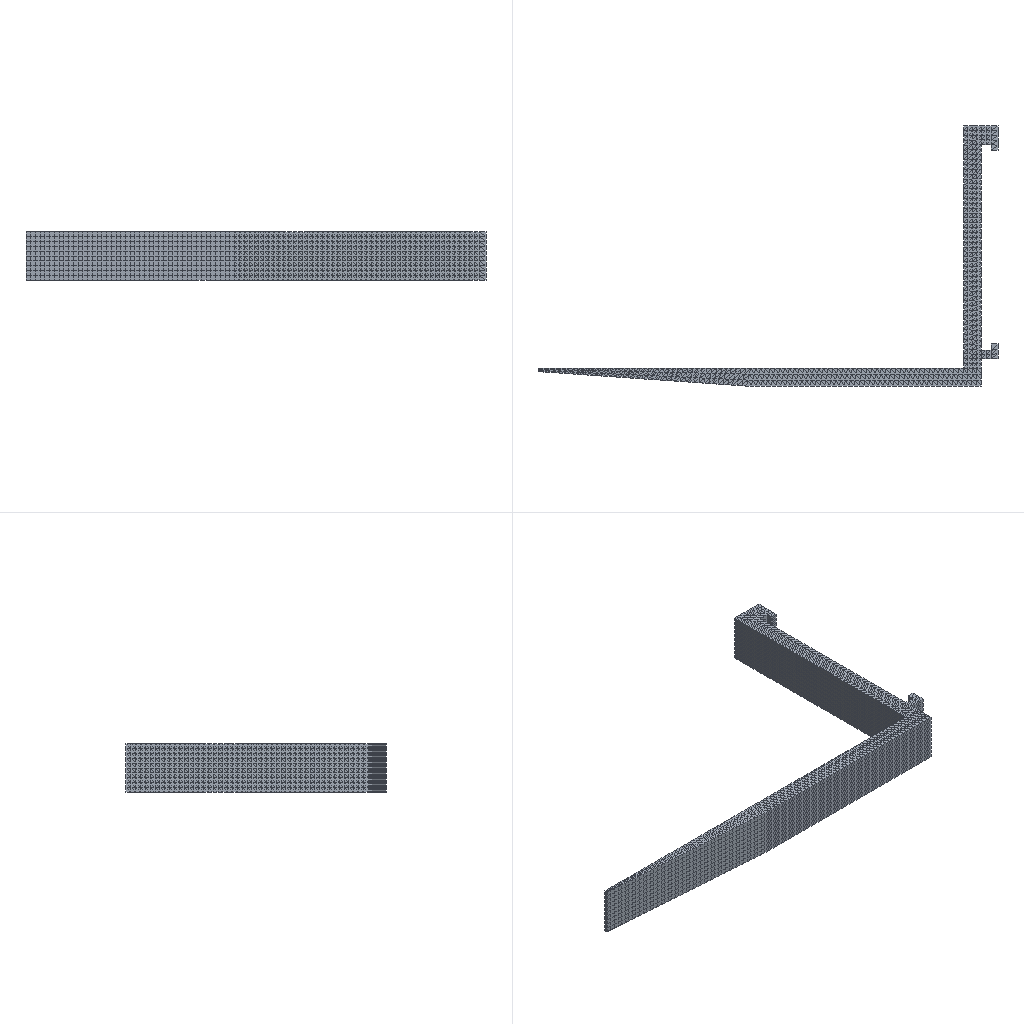Simulation study | abaqus
Set-up summary:
category,name,step,type,value,unit,region
solver,abaqus,,Abaqus/CAE 2024
units,mm-N-s-tonne (MPa),,inferred,E=240000 density=1.8e-09
analysis,Step-1,,dynamic explicit,nlgeom=True; time_period=1
mesh,nodes,,,7150
mesh,elements,,,8982
element_type,C3D8R,,,4960
element_type,S4R,,,4022
material,Material-CFRP,,E,240000
material,Material-CFRP,,nu,0.25
material,Material-CFRP,,density,1.8e-09
material,Material-CFRP,,behaviors,damage initiation; damage evolution; elastic lamina
material,Material-foam,,density,5.1e-11
section,Material-foam,,solid section,,,Set-31
section,,,shell section,0.2,,CompositeLayup-1-1
section,,,shell section,0.2,,CompositeLayup-2-1
load,Load-1,Step-1,pressure,0.1,,Surf-2
bc,BC-1,initial,encastre,[dofs=ENCASTRE],,Set-2
contact,Int-1,initial,general contact,interaction=IntProp-1; friction=0.15; behavior=hard
Abaqus input file, long lists of numbers shortened:
*Heading
** Job name: deck Model name: 0413
** Generated by: Abaqus/CAE 2024
*Preprint, echo=NO, model=NO, history=NO, contact=NO
**
** PARTS
**
*Part, name=huocha
*End Part
**
**
** ASSEMBLY
**
*Assembly, name=Assembly
**
*Instance, name=huocha-1, part=huocha
*Node
      1,        1118.,         598.,         120.
      2,        1118.,         598.,           0.
** (7148 more lines like these left out)
*Element, type=C3D8R
 1,   90,  861, 4172,  855,    1,   45,  837,   64
 2,  861,  862, 4173, 4172,   45,   46,  838,  837
** (4958 more lines like these left out)
*Element, type=S4R
4961,   5, 172,  18,  17
4962,  96, 173, 172,   5
** (4020 more lines like these left out)
*Nset, nset=_PickedSet5, internal
    1,    2,    3,    4,    5,    6,    7,    8,    9,   10,   11,   12,   13,   14,   15,   16
   17,   18,   19,   20,   21,   22,   23,   26,   27,   28,   29,   30,   31,   32,   33,   34
** (139 more lines like these left out)
*Elset, elset=_PickedSet5, internal
 4974, 4975, 4976, 4977, 4978, 4979, 4980, 4981, 4982, 4983, 4984, 4985, 4986, 4987, 4988, 4989
 4990, 4991, 4992, 4993, 4994, 4995, 4996, 4997, 4998, 4999, 5000, 5001, 5002, 5003, 5011, 5012
** (121 more lines like these left out)
*Nset, nset=_PickedSet6, internal
    1,    2,    3,    4,    5,    6,    7,    8,    9,   10,   11,   12,   13,   14,   15,   16
   17,   18,   19,   20,   21,   22,   23,   26,   27,   28,   29,   30,   31,   32,   33,   34
** (139 more lines like these left out)
*Elset, elset=_PickedSet6, internal
 4974, 4975, 4976, 4977, 4978, 4979, 4980, 4981, 4982, 4983, 4984, 4985, 4986, 4987, 4988, 4989
 4990, 4991, 4992, 4993, 4994, 4995, 4996, 4997, 4998, 4999, 5000, 5001, 5002, 5003, 5011, 5012
** (121 more lines like these left out)
*Nset, nset=_PickedSet7, internal
    1,    2,    3,    4,    5,    6,    7,    8,    9,   10,   11,   12,   13,   14,   15,   16
   17,   18,   19,   20,   21,   22,   23,   26,   27,   28,   29,   30,   31,   32,   33,   34
** (139 more lines like these left out)
*Elset, elset=_PickedSet7, internal
 4974, 4975, 4976, 4977, 4978, 4979, 4980, 4981, 4982, 4983, 4984, 4985, 4986, 4987, 4988, 4989
 4990, 4991, 4992, 4993, 4994, 4995, 4996, 4997, 4998, 4999, 5000, 5001, 5002, 5003, 5011, 5012
** (121 more lines like these left out)
*Nset, nset=_PickedSet8, internal
    1,    2,    3,    4,    5,    6,    7,    8,    9,   10,   11,   12,   13,   14,   15,   16
   17,   18,   19,   20,   21,   22,   23,   26,   27,   28,   29,   30,   31,   32,   33,   34
** (139 more lines like these left out)
*Elset, elset=_PickedSet8, internal
 4974, 4975, 4976, 4977, 4978, 4979, 4980, 4981, 4982, 4983, 4984, 4985, 4986, 4987, 4988, 4989
 4990, 4991, 4992, 4993, 4994, 4995, 4996, 4997, 4998, 4999, 5000, 5001, 5002, 5003, 5011, 5012
** (121 more lines like these left out)
*Nset, nset=_PickedSet9, internal
    1,    2,    3,    4,    5,    6,    7,    8,    9,   10,   11,   12,   13,   14,   15,   16
   17,   18,   19,   20,   21,   22,   23,   26,   27,   28,   29,   30,   31,   32,   33,   34
** (139 more lines like these left out)
*Elset, elset=_PickedSet9, internal
 4974, 4975, 4976, 4977, 4978, 4979, 4980, 4981, 4982, 4983, 4984, 4985, 4986, 4987, 4988, 4989
 4990, 4991, 4992, 4993, 4994, 4995, 4996, 4997, 4998, 4999, 5000, 5001, 5002, 5003, 5011, 5012
** (121 more lines like these left out)
*Nset, nset=_PickedSet10, internal
    1,    2,    3,    4,    5,    6,    7,    8,    9,   10,   11,   12,   13,   14,   15,   16
   17,   18,   19,   20,   21,   22,   23,   26,   27,   28,   29,   30,   31,   32,   33,   34
** (139 more lines like these left out)
*Elset, elset=_PickedSet10, internal
 4974, 4975, 4976, 4977, 4978, 4979, 4980, 4981, 4982, 4983, 4984, 4985, 4986, 4987, 4988, 4989
 4990, 4991, 4992, 4993, 4994, 4995, 4996, 4997, 4998, 4999, 5000, 5001, 5002, 5003, 5011, 5012
** (121 more lines like these left out)
*Nset, nset=_PickedSet11, internal
    1,    2,    3,    4,    5,    6,    7,    8,    9,   10,   11,   12,   13,   14,   15,   16
   17,   18,   19,   20,   21,   22,   23,   26,   27,   28,   29,   30,   31,   32,   33,   34
** (139 more lines like these left out)
*Elset, elset=_PickedSet11, internal
 4974, 4975, 4976, 4977, 4978, 4979, 4980, 4981, 4982, 4983, 4984, 4985, 4986, 4987, 4988, 4989
 4990, 4991, 4992, 4993, 4994, 4995, 4996, 4997, 4998, 4999, 5000, 5001, 5002, 5003, 5011, 5012
** (121 more lines like these left out)
*Nset, nset=_PickedSet12, internal
    1,    2,    3,    4,    5,    6,    7,    8,    9,   10,   11,   12,   13,   14,   15,   16
   17,   18,   19,   20,   21,   22,   23,   26,   27,   28,   29,   30,   31,   32,   33,   34
** (139 more lines like these left out)
*Elset, elset=_PickedSet12, internal
 4974, 4975, 4976, 4977, 4978, 4979, 4980, 4981, 4982, 4983, 4984, 4985, 4986, 4987, 4988, 4989
 4990, 4991, 4992, 4993, 4994, 4995, 4996, 4997, 4998, 4999, 5000, 5001, 5002, 5003, 5011, 5012
** (121 more lines like these left out)
*Nset, nset=_PickedSet13, internal
    1,    2,    3,    4,    5,    6,    7,    8,    9,   10,   11,   12,   13,   14,   15,   16
   17,   18,   19,   20,   21,   22,   23,   26,   27,   28,   29,   30,   31,   32,   33,   34
** (139 more lines like these left out)
*Elset, elset=_PickedSet13, internal
 4974, 4975, 4976, 4977, 4978, 4979, 4980, 4981, 4982, 4983, 4984, 4985, 4986, 4987, 4988, 4989
 4990, 4991, 4992, 4993, 4994, 4995, 4996, 4997, 4998, 4999, 5000, 5001, 5002, 5003, 5011, 5012
** (121 more lines like these left out)
*Nset, nset=_PickedSet14, internal
    1,    2,    3,    4,    5,    6,    7,    8,    9,   10,   11,   12,   13,   14,   15,   16
   17,   18,   19,   20,   21,   22,   23,   26,   27,   28,   29,   30,   31,   32,   33,   34
** (139 more lines like these left out)
*Elset, elset=_PickedSet14, internal
 4974, 4975, 4976, 4977, 4978, 4979, 4980, 4981, 4982, 4983, 4984, 4985, 4986, 4987, 4988, 4989
 4990, 4991, 4992, 4993, 4994, 4995, 4996, 4997, 4998, 4999, 5000, 5001, 5002, 5003, 5011, 5012
** (121 more lines like these left out)
*Nset, nset=_PickedSet15, internal
    1,    2,    3,    4,    5,    6,    7,    8,    9,   10,   11,   12,   13,   14,   15,   16
   17,   18,   19,   20,   21,   22,   23,   24,   25,   26,   27,   28,   29,   30,   31,   32
** (194 more lines like these left out)
*Elset, elset=_PickedSet15, internal, generate
 4961,  7912,     1
*Nset, nset=_PickedSet16, internal
    1,    2,    3,    4,    5,    6,    7,    8,    9,   10,   11,   12,   13,   14,   15,   16
   17,   18,   19,   20,   21,   22,   23,   24,   25,   26,   27,   28,   29,   30,   31,   32
** (194 more lines like these left out)
*Elset, elset=_PickedSet16, internal, generate
 4961,  7912,     1
*Nset, nset=_PickedSet17, internal
    1,    2,    3,    4,    5,    6,    7,    8,    9,   10,   11,   12,   13,   14,   15,   16
   17,   18,   19,   20,   21,   22,   23,   24,   25,   26,   27,   28,   29,   30,   31,   32
** (194 more lines like these left out)
*Elset, elset=_PickedSet17, internal, generate
 4961,  7912,     1
*Nset, nset=_PickedSet18, internal
    1,    2,    3,    4,    5,    6,    7,    8,    9,   10,   11,   12,   13,   14,   15,   16
   17,   18,   19,   20,   21,   22,   23,   24,   25,   26,   27,   28,   29,   30,   31,   32
** (194 more lines like these left out)
*Elset, elset=_PickedSet18, internal, generate
 4961,  7912,     1
*Nset, nset=_PickedSet19, internal
    1,    2,    3,    4,    5,    6,    7,    8,    9,   10,   11,   12,   13,   14,   15,   16
   17,   18,   19,   20,   21,   22,   23,   24,   25,   26,   27,   28,   29,   30,   31,   32
** (194 more lines like these left out)
*Elset, elset=_PickedSet19, internal, generate
 4961,  7912,     1
*Nset, nset=_PickedSet20, internal
    1,    2,    3,    4,    5,    6,    7,    8,    9,   10,   11,   12,   13,   14,   15,   16
   17,   18,   19,   20,   21,   22,   23,   24,   25,   26,   27,   28,   29,   30,   31,   32
** (194 more lines like these left out)
*Elset, elset=_PickedSet20, internal, generate
 4961,  7912,     1
*Nset, nset=_PickedSet21, internal
    1,    2,    3,    4,    5,    6,    7,    8,    9,   10,   11,   12,   13,   14,   15,   16
   17,   18,   19,   20,   21,   22,   23,   24,   25,   26,   27,   28,   29,   30,   31,   32
** (194 more lines like these left out)
*Elset, elset=_PickedSet21, internal, generate
 4961,  7912,     1
*Nset, nset=_PickedSet22, internal
    1,    2,    3,    4,    5,    6,    7,    8,    9,   10,   11,   12,   13,   14,   15,   16
   17,   18,   19,   20,   21,   22,   23,   24,   25,   26,   27,   28,   29,   30,   31,   32
** (194 more lines like these left out)
*Elset, elset=_PickedSet22, internal, generate
 4961,  7912,     1
*Nset, nset=_PickedSet23, internal
    1,    2,    3,    4,    5,    6,    7,    8,    9,   10,   11,   12,   13,   14,   15,   16
   17,   18,   19,   20,   21,   22,   23,   24,   25,   26,   27,   28,   29,   30,   31,   32
** (194 more lines like these left out)
*Elset, elset=_PickedSet23, internal, generate
 4961,  7912,     1
*Nset, nset=_PickedSet24, internal
    1,    2,    3,    4,    5,    6,    7,    8,    9,   10,   11,   12,   13,   14,   15,   16
   17,   18,   19,   20,   21,   22,   23,   24,   25,   26,   27,   28,   29,   30,   31,   32
** (194 more lines like these left out)
*Elset, elset=_PickedSet24, internal, generate
 4961,  7912,     1
*Nset, nset=_PickedSet27, internal
    5,    6,    7,    8,   11,   12,   13,   14,   15,   16,   17,   20,   23,   24,   25,   26
   27,   28,   31,   34,   43,   44,   65,   66,   67,   68,   69,   70,   71,   72,   73,   75
** (70 more lines like these left out)
*Elset, elset=_PickedSet27, internal, generate
 7913,  8902,     1
*Nset, nset=_PickedSet28, internal
    5,    6,    7,    8,   11,   12,   13,   14,   15,   16,   17,   20,   23,   24,   25,   26
   27,   28,   31,   34,   43,   44,   65,   66,   67,   68,   69,   70,   71,   72,   73,   75
** (70 more lines like these left out)
*Elset, elset=_PickedSet28, internal, generate
 7913,  8902,     1
*Nset, nset=_PickedSet29, internal
    5,    6,    7,    8,   11,   12,   13,   14,   15,   16,   17,   20,   23,   24,   25,   26
   27,   28,   31,   34,   43,   44,   65,   66,   67,   68,   69,   70,   71,   72,   73,   75
** (70 more lines like these left out)
*Elset, elset=_PickedSet29, internal, generate
 7913,  8902,     1
*Nset, nset=_PickedSet30, internal
    5,    6,    7,    8,   11,   12,   13,   14,   15,   16,   17,   20,   23,   24,   25,   26
   27,   28,   31,   34,   43,   44,   65,   66,   67,   68,   69,   70,   71,   72,   73,   75
** (70 more lines like these left out)
*Elset, elset=_PickedSet30, internal, generate
 7913,  8902,     1
*Nset, nset=_PickedSet31, internal
    5,    6,    7,    8,   11,   12,   13,   14,   15,   16,   17,   20,   23,   24,   25,   26
   27,   28,   31,   34,   43,   44,   65,   66,   67,   68,   69,   70,   71,   72,   73,   75
** (70 more lines like these left out)
*Elset, elset=_PickedSet31, internal, generate
 7913,  8902,     1
*Nset, nset=_PickedSet32, internal
    5,    6,    7,    8,   11,   12,   13,   14,   15,   16,   17,   20,   23,   24,   25,   26
   27,   28,   31,   34,   43,   44,   65,   66,   67,   68,   69,   70,   71,   72,   73,   75
** (70 more lines like these left out)
*Elset, elset=_PickedSet32, internal, generate
 7913,  8902,     1
*Nset, nset=_PickedSet33, internal
    5,    6,    7,    8,   11,   12,   13,   14,   15,   16,   17,   20,   23,   24,   25,   26
   27,   28,   31,   34,   43,   44,   65,   66,   67,   68,   69,   70,   71,   72,   73,   75
** (70 more lines like these left out)
*Elset, elset=_PickedSet33, internal, generate
 7913,  8902,     1
*Nset, nset=_PickedSet34, internal
    5,    6,    7,    8,   11,   12,   13,   14,   15,   16,   17,   20,   23,   24,   25,   26
   27,   28,   31,   34,   43,   44,   65,   66,   67,   68,   69,   70,   71,   72,   73,   75
** (70 more lines like these left out)
*Elset, elset=_PickedSet34, internal, generate
 7913,  8902,     1
*Nset, nset=_PickedSet35, internal
    5,    6,    7,    8,   11,   12,   13,   14,   15,   16,   17,   20,   23,   24,   25,   26
   27,   28,   31,   34,   43,   44,   65,   66,   67,   68,   69,   70,   71,   72,   73,   75
** (70 more lines like these left out)
*Elset, elset=_PickedSet35, internal, generate
 7913,  8902,     1
*Nset, nset=_PickedSet36, internal
    5,    6,    7,    8,   11,   12,   13,   14,   15,   16,   17,   20,   23,   24,   25,   26
   27,   28,   31,   34,   43,   44,   65,   66,   67,   68,   69,   70,   71,   72,   73,   75
** (70 more lines like these left out)
*Elset, elset=_PickedSet36, internal, generate
 7913,  8902,     1
*Nset, nset=Set-31, generate
    1,  7150,     1
*Elset, elset=Set-31, generate
    1,  4960,     1
*Nset, nset=_Skin-1, internal
    1,    2,    3,    4,    5,    6,    7,    8,    9,   10,   11,   12,   13,   14,   15,   16
   17,   18,   19,   20,   21,   22,   23,   24,   25,   26,   27,   28,   29,   30,   31,   32
** (194 more lines like these left out)
*Elset, elset=_Skin-1, internal, generate
 4961,  7912,     1
*Nset, nset=_PickedSet42, internal
    1,    2,    3,    4,    5,    6,    7,    8,    9,   10,   11,   12,   13,   14,   15,   16
   17,   18,   19,   20,   21,   22,   23,   24,   25,   26,   27,   28,   29,   30,   31,   32
** (189 more lines like these left out)
*Elset, elset=_PickedSet42, internal
 4961, 4962, 4963, 4964, 4965, 4966, 4967, 4968, 4969, 4970, 4971, 4972, 4973, 4984, 4985, 4986
 4987, 4988, 4989, 4990, 4991, 4992, 4993, 4994, 4995, 4996, 4997, 4998, 4999, 5000, 5001, 5002
** (178 more lines like these left out)
*Nset, nset=_PickedSet43, internal
    1,    2,    3,    4,    5,    6,    7,    8,    9,   10,   11,   12,   13,   14,   15,   16
   17,   18,   19,   20,   21,   22,   23,   24,   25,   26,   27,   28,   29,   30,   31,   32
** (189 more lines like these left out)
*Elset, elset=_PickedSet43, internal
 4961, 4962, 4963, 4964, 4965, 4966, 4967, 4968, 4969, 4970, 4971, 4972, 4973, 4984, 4985, 4986
 4987, 4988, 4989, 4990, 4991, 4992, 4993, 4994, 4995, 4996, 4997, 4998, 4999, 5000, 5001, 5002
** (178 more lines like these left out)
*Nset, nset=_PickedSet44, internal
    1,    2,    3,    4,    5,    6,    7,    8,    9,   10,   11,   12,   13,   14,   15,   16
   17,   18,   19,   20,   21,   22,   23,   24,   25,   26,   27,   28,   29,   30,   31,   32
** (189 more lines like these left out)
*Elset, elset=_PickedSet44, internal
 4961, 4962, 4963, 4964, 4965, 4966, 4967, 4968, 4969, 4970, 4971, 4972, 4973, 4984, 4985, 4986
 4987, 4988, 4989, 4990, 4991, 4992, 4993, 4994, 4995, 4996, 4997, 4998, 4999, 5000, 5001, 5002
** (178 more lines like these left out)
*Nset, nset=_PickedSet45, internal
    1,    2,    3,    4,    5,    6,    7,    8,    9,   10,   11,   12,   13,   14,   15,   16
   17,   18,   19,   20,   21,   22,   23,   24,   25,   26,   27,   28,   29,   30,   31,   32
** (189 more lines like these left out)
*Elset, elset=_PickedSet45, internal
 4961, 4962, 4963, 4964, 4965, 4966, 4967, 4968, 4969, 4970, 4971, 4972, 4973, 4984, 4985, 4986
 4987, 4988, 4989, 4990, 4991, 4992, 4993, 4994, 4995, 4996, 4997, 4998, 4999, 5000, 5001, 5002
** (178 more lines like these left out)
*Nset, nset=_PickedSet46, internal
    1,    2,    3,    4,    5,    6,    7,    8,    9,   10,   11,   12,   13,   14,   15,   16
   17,   18,   19,   20,   21,   22,   23,   24,   25,   26,   27,   28,   29,   30,   31,   32
** (189 more lines like these left out)
*Elset, elset=_PickedSet46, internal
 4961, 4962, 4963, 4964, 4965, 4966, 4967, 4968, 4969, 4970, 4971, 4972, 4973, 4984, 4985, 4986
 4987, 4988, 4989, 4990, 4991, 4992, 4993, 4994, 4995, 4996, 4997, 4998, 4999, 5000, 5001, 5002
** (178 more lines like these left out)
*Nset, nset=_PickedSet47, internal
    1,    2,    3,    4,    5,    6,    7,    8,    9,   10,   11,   12,   13,   14,   15,   16
   17,   18,   19,   20,   21,   22,   23,   24,   25,   26,   27,   28,   29,   30,   31,   32
** (189 more lines like these left out)
*Elset, elset=_PickedSet47, internal
 4961, 4962, 4963, 4964, 4965, 4966, 4967, 4968, 4969, 4970, 4971, 4972, 4973, 4984, 4985, 4986
 4987, 4988, 4989, 4990, 4991, 4992, 4993, 4994, 4995, 4996, 4997, 4998, 4999, 5000, 5001, 5002
** (178 more lines like these left out)
*Nset, nset=_PickedSet48, internal
    1,    2,    3,    4,    5,    6,    7,    8,    9,   10,   11,   12,   13,   14,   15,   16
   17,   18,   19,   20,   21,   22,   23,   24,   25,   26,   27,   28,   29,   30,   31,   32
** (189 more lines like these left out)
*Elset, elset=_PickedSet48, internal
 4961, 4962, 4963, 4964, 4965, 4966, 4967, 4968, 4969, 4970, 4971, 4972, 4973, 4984, 4985, 4986
 4987, 4988, 4989, 4990, 4991, 4992, 4993, 4994, 4995, 4996, 4997, 4998, 4999, 5000, 5001, 5002
** (178 more lines like these left out)
*Nset, nset=_PickedSet49, internal
    1,    2,    3,    4,    5,    6,    7,    8,    9,   10,   11,   12,   13,   14,   15,   16
   17,   18,   19,   20,   21,   22,   23,   24,   25,   26,   27,   28,   29,   30,   31,   32
** (189 more lines like these left out)
*Elset, elset=_PickedSet49, internal
 4961, 4962, 4963, 4964, 4965, 4966, 4967, 4968, 4969, 4970, 4971, 4972, 4973, 4984, 4985, 4986
 4987, 4988, 4989, 4990, 4991, 4992, 4993, 4994, 4995, 4996, 4997, 4998, 4999, 5000, 5001, 5002
** (178 more lines like these left out)
*Nset, nset=_PickedSet50, internal
    1,    2,    3,    4,    5,    6,    7,    8,    9,   10,   11,   12,   13,   14,   15,   16
   17,   18,   19,   20,   21,   22,   23,   24,   25,   26,   27,   28,   29,   30,   31,   32
** (189 more lines like these left out)
*Elset, elset=_PickedSet50, internal
 4961, 4962, 4963, 4964, 4965, 4966, 4967, 4968, 4969, 4970, 4971, 4972, 4973, 4984, 4985, 4986
 4987, 4988, 4989, 4990, 4991, 4992, 4993, 4994, 4995, 4996, 4997, 4998, 4999, 5000, 5001, 5002
** (178 more lines like these left out)
*Nset, nset=_PickedSet51, internal
    1,    2,    3,    4,    5,    6,    7,    8,    9,   10,   11,   12,   13,   14,   15,   16
   17,   18,   19,   20,   21,   22,   23,   24,   25,   26,   27,   28,   29,   30,   31,   32
** (189 more lines like these left out)
*Elset, elset=_PickedSet51, internal
 4961, 4962, 4963, 4964, 4965, 4966, 4967, 4968, 4969, 4970, 4971, 4972, 4973, 4984, 4985, 4986
 4987, 4988, 4989, 4990, 4991, 4992, 4993, 4994, 4995, 4996, 4997, 4998, 4999, 5000, 5001, 5002
** (178 more lines like these left out)
*Nset, nset=_PickedSet53, internal
    5,    6,    7,    8,   11,   12,   13,   14,   15,   16,   17,   20,   23,   24,   25,   26
   27,   28,   31,   34,   43,   44,   65,   66,   67,   68,   69,   70,   71,   72,   73,   75
** (70 more lines like these left out)
*Elset, elset=_PickedSet53, internal, generate
 7913,  8902,     1
*Nset, nset=_PickedSet54, internal
    5,    6,    7,    8,   11,   12,   13,   14,   15,   16,   17,   20,   23,   24,   25,   26
   27,   28,   31,   34,   43,   44,   65,   66,   67,   68,   69,   70,   71,   72,   73,   75
** (70 more lines like these left out)
*Elset, elset=_PickedSet54, internal, generate
 7913,  8902,     1
*Nset, nset=_PickedSet55, internal
    5,    6,    7,    8,   11,   12,   13,   14,   15,   16,   17,   20,   23,   24,   25,   26
   27,   28,   31,   34,   43,   44,   65,   66,   67,   68,   69,   70,   71,   72,   73,   75
** (70 more lines like these left out)
*Elset, elset=_PickedSet55, internal, generate
 7913,  8902,     1
*Nset, nset=_PickedSet56, internal
    5,    6,    7,    8,   11,   12,   13,   14,   15,   16,   17,   20,   23,   24,   25,   26
   27,   28,   31,   34,   43,   44,   65,   66,   67,   68,   69,   70,   71,   72,   73,   75
** (70 more lines like these left out)
*Elset, elset=_PickedSet56, internal, generate
 7913,  8902,     1
*Nset, nset=_PickedSet57, internal
    5,    6,    7,    8,   11,   12,   13,   14,   15,   16,   17,   20,   23,   24,   25,   26
   27,   28,   31,   34,   43,   44,   65,   66,   67,   68,   69,   70,   71,   72,   73,   75
** (70 more lines like these left out)
*Elset, elset=_PickedSet57, internal, generate
 7913,  8902,     1
*Nset, nset=_PickedSet58, internal
    5,    6,    7,    8,   11,   12,   13,   14,   15,   16,   17,   20,   23,   24,   25,   26
   27,   28,   31,   34,   43,   44,   65,   66,   67,   68,   69,   70,   71,   72,   73,   75
** (70 more lines like these left out)
*Elset, elset=_PickedSet58, internal, generate
 7913,  8902,     1
*Nset, nset=_PickedSet59, internal
    5,    6,    7,    8,   11,   12,   13,   14,   15,   16,   17,   20,   23,   24,   25,   26
   27,   28,   31,   34,   43,   44,   65,   66,   67,   68,   69,   70,   71,   72,   73,   75
** (70 more lines like these left out)
*Elset, elset=_PickedSet59, internal, generate
 7913,  8902,     1
*Nset, nset=_PickedSet60, internal
    5,    6,    7,    8,   11,   12,   13,   14,   15,   16,   17,   20,   23,   24,   25,   26
   27,   28,   31,   34,   43,   44,   65,   66,   67,   68,   69,   70,   71,   72,   73,   75
** (70 more lines like these left out)
*Elset, elset=_PickedSet60, internal, generate
 7913,  8902,     1
*Nset, nset=_PickedSet61, internal
    5,    6,    7,    8,   11,   12,   13,   14,   15,   16,   17,   20,   23,   24,   25,   26
   27,   28,   31,   34,   43,   44,   65,   66,   67,   68,   69,   70,   71,   72,   73,   75
** (70 more lines like these left out)
*Elset, elset=_PickedSet61, internal, generate
 7913,  8902,     1
*Nset, nset=_PickedSet62, internal
    5,    6,    7,    8,   11,   12,   13,   14,   15,   16,   17,   20,   23,   24,   25,   26
   27,   28,   31,   34,   43,   44,   65,   66,   67,   68,   69,   70,   71,   72,   73,   75
** (70 more lines like these left out)
*Elset, elset=_PickedSet62, internal, generate
 7913,  8902,     1
*Nset, nset=_Skin-2, internal
    5,    6,    7,    8,   11,   12,   13,   14,   15,   16,   17,   20,   23,   24,   25,   26
   27,   28,   31,   34,   43,   44,   65,   66,   67,   68,   69,   70,   71,   72,   73,   75
** (70 more lines like these left out)
*Elset, elset=_Skin-2, internal, generate
 7913,  8902,     1
*Nset, nset=_Skin-3, internal
   18,   19,   21,   22,   29,   30,   32,   33,  141,  142,  143,  144,  145,  146,  147,  148
  149,  159,  160,  161,  162,  163,  164,  165,  166,  167,  168,  169,  170,  171,  172,  173
** (5 more lines like these left out)
*Elset, elset=_Skin-3, internal, generate
 8903,  8982,     1
** Section: Section-1
*Solid Section, elset=Set-31, material=Material-foam
,
*Orientation, name=Ori-1
1., 0., 0., 0., 1., 0.
3, 0.
** Region: (CompositeLayup-1-1: Generated From Layup)
*Elset, elset=CompositeLayup-1-1, generate
 4961,  7912,     1
** Section: CompositeLayup-1-1
*Shell Section, elset=CompositeLayup-1-1, composite, orientation=Ori-1, layup=CompositeLayup-1
0.2, 3, Material-CFRP, 0., 层-1
0.2, 3, Material-CFRP, 45., 层-2
0.2, 3, Material-CFRP, 90., 层-3
0.2, 3, Material-CFRP, -45., 层-4
0.2, 3, Material-CFRP, 0., 层-5
0.2, 3, Material-CFRP, 0., 层-6
0.2, 3, Material-CFRP, -45., 层-7
0.2, 3, Material-CFRP, 90., 层-8
0.2, 3, Material-CFRP, 45., 层-9
0.2, 3, Material-CFRP, 0., 层-10
*Orientation, name=Ori-2
          0.,           1.,           0.,           0.,           0.,          -1.
3, 0.
** Region: (CompositeLayup-2-1: Generated From Layup)
*Elset, elset=CompositeLayup-2-1, generate
 7913,  8982,     1
** Section: CompositeLayup-2-1
*Shell Section, elset=CompositeLayup-2-1, composite, orientation=Ori-2, layup=CompositeLayup-2
0.2, 3, Material-CFRP, 0., 层-1
0.2, 3, Material-CFRP, 45., 层-2
0.2, 3, Material-CFRP, 90., 层-3
0.2, 3, Material-CFRP, -45., 层-4
0.2, 3, Material-CFRP, 0., 层-5
0.2, 3, Material-CFRP, 0., 层-6
0.2, 3, Material-CFRP, -45., 层-7
0.2, 3, Material-CFRP, 90., 层-8
0.2, 3, Material-CFRP, 45., 层-9
0.2, 3, Material-CFRP, 0., 层-10
*End Instance
**
*Nset, nset=Set-2, instance=huocha-1
   18,   19,   21,   22,   29,   30,   32,   33,  141,  142,  143,  144,  145,  146,  147,  148
  149,  159,  160,  161,  162,  163,  164,  165,  166,  167,  168,  169,  170,  171,  172,  173
** (5 more lines like these left out)
*Elset, elset=Set-2, instance=huocha-1
  121,  122,  123,  124,  125,  126,  127,  128,  129,  130,  131,  132,  133,  134,  135,  136
  137,  138,  139,  140,  141,  142,  143,  144,  145,  146,  147,  148,  149,  150,  151,  152
** (3 more lines like these left out)
*Elset, elset=_Surf-2_S3, internal, instance=huocha-1
 3641, 3642, 3643, 3644, 3645, 3646, 3647, 3648, 3649, 3650, 3671, 3672, 3673, 3674, 3675, 3676
 3677, 3678, 3679, 3680, 3701, 3702, 3703, 3704, 3705, 3706, 3707, 3708, 3709, 3710, 3731, 3732
** (26 more lines like these left out)
*Elset, elset=_Surf-2_S2, internal, instance=huocha-1, generate
 2201,  2640,     1
*Surface, type=ELEMENT, name=Surf-2
_Surf-2_S3, S3
_Surf-2_S2, S2
*End Assembly
*Amplitude, name=Amp-1
             0.,              0.,              1.,              1.
**
** MATERIALS
**
*Material, name=Material-CFRP
*Damage Initiation, criterion=HASHIN
2500.,2500.,  50., 150., 100.,  60.
*Damage Evolution, type=ENERGY
150.,100.,  1., 10.
*Density
 1.8e-09,
*Elastic, type=LAMINA
240000.,15000.,  0.25,30000.,30000., 7000.
*Material, name=Material-foam
*Density
 5.1e-11,
*Low Density Foam, tension cutoff=202.
0.0001, 0.005, 2.
*Uniaxial Test Data, direction=TENSION
  0.,    0.,    0.
 2.2, 0.021,    0.
*Uniaxial Test Data, direction=COMPRESSION
    0.,      0.,      0.
 0.402, 0.00448,      0.
 0.894,  0.0112,      0.
  1.39,  0.0202,      0.
  1.77,  0.0269,      0.
  1.97,  0.0359,      0.
  2.06,  0.0471,      0.
   2.1,   0.065,      0.
  2.01,   0.083,      0.
   1.9,  0.0987,      0.
  1.88,   0.117,      0.
  1.88,    0.17,      0.
  1.97,   0.287,      0.
  1.92,   0.359,      0.
  1.92,   0.471,      0.
  1.94,   0.581,      0.
  1.97,   0.605,      0.
  2.03,   0.621,      0.
  2.15,   0.637,      0.
  2.48,   0.664,      0.
  2.91,   0.695,      0.
  3.26,    0.72,      0.
  3.71,   0.742,      0.
   4.2,   0.765,      0.
  4.87,   0.785,      0.
  5.63,   0.812,      0.
  6.17,   0.834,      0.
  6.84,   0.848,      0.
  7.98,   0.863,      0.
**
** INTERACTION PROPERTIES
**
*Surface Interaction, name=IntProp-1
*Friction
 0.15,
*Surface Behavior, pressure-overclosure=HARD
**
** BOUNDARY CONDITIONS
**
** Name: BC-1 Type: Symmetry/Antisymmetry/Encastre
*Boundary
Set-2, ENCASTRE
**
** INTERACTIONS
**
** Interaction: Int-1
*Contact, op=NEW
*Contact Inclusions, ALL EXTERIOR
*Contact Property Assignment
 ,  , IntProp-1
** ----------------------------------------------------------------
**
** STEP: Step-1
**
*Step, name=Step-1, nlgeom=YES
*Dynamic, Explicit
, 1.
*Bulk Viscosity
0.06, 1.2
** Mass Scaling: Semi-Automatic
**               Whole Model
*Fixed Mass Scaling, factor=10000.
**
** LOADS
**
** Name: Load-1   Type: Pressure
*Dsload, amplitude=Amp-1
Surf-2, P, 0.1
**
** OUTPUT REQUESTS
**
*Restart, write, number interval=1, time marks=NO
**
** FIELD OUTPUT: F-Output-1
**
*Output, field, variable=PRESELECT
**
** HISTORY OUTPUT: H-Output-1
**
*Output, history, variable=PRESELECT, frequency=1
*End Step
Results summary:
result,odb.job_status,,,JOB_STATUS_COMPLETED_SUCCESSFULLY,"consistent, unstated (Abaqus has no unit system)"
result,steps[0].procedure,Step-1,,"*DYNAMIC, EXPLICIT","consistent, unstated (Abaqus has no unit system)"
result,steps[0].time_period,Step-1,,1,"consistent, unstated (Abaqus has no unit system)"
result,steps[0].n_frames,Step-1,,21,"consistent, unstated (Abaqus has no unit system)"
result,steps[0].last_frame.id,Step-1,,45100,"consistent, unstated (Abaqus has no unit system)"
result,steps[0].last_frame.value,Step-1,,1,"consistent, unstated (Abaqus has no unit system)"
result,steps[0].last_frame.description,Step-1,,Increment     45100: Step Time =    1.000,"consistent, unstated (Abaqus has no unit system)"
result,steps[0].completed,Step-1,,True,"consistent, unstated (Abaqus has no unit system)"
result,steps[0].max_U_magnitude,Step-1,,189.118,"consistent, unstated (Abaqus has no unit system)"
result,steps[0].max_S_mises,Step-1,,2390.72,"consistent, unstated (Abaqus has no unit system)"
result,steps[0].RF_sum[1],Step-1,,2244.18,"consistent, unstated (Abaqus has no unit system)"
result,steps[0].RF_sum[2],Step-1,,-84.015,"consistent, unstated (Abaqus has no unit system)"
result,steps[0].RF_sum[3],Step-1,,-3867.65,"consistent, unstated (Abaqus has no unit system)"
result,steps[0].diagnostic.n_increments,Step-1,,21,"consistent, unstated (Abaqus has no unit system)"